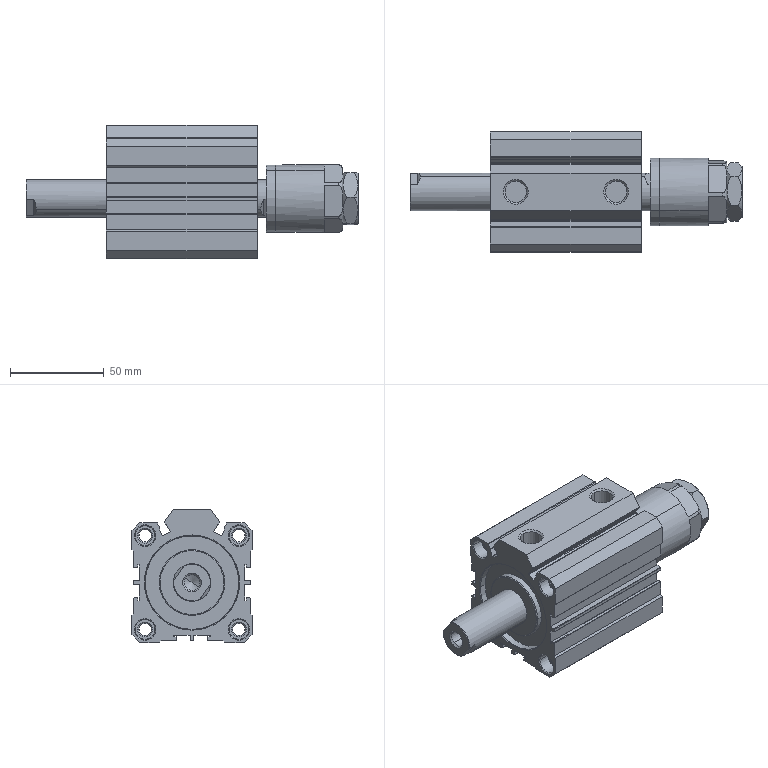Part | SolidWorks | 4 solids | 358 faces | box 177 x 64 x 71 mm | volume 281305 mm3 | plane 131 | cylinder 128 | cone 93 | spline 6 | commonest cylinder face diameters 0.4 x35 6.647 x16 10.5 x16 0.8 x15 6.5 x8 20 x8